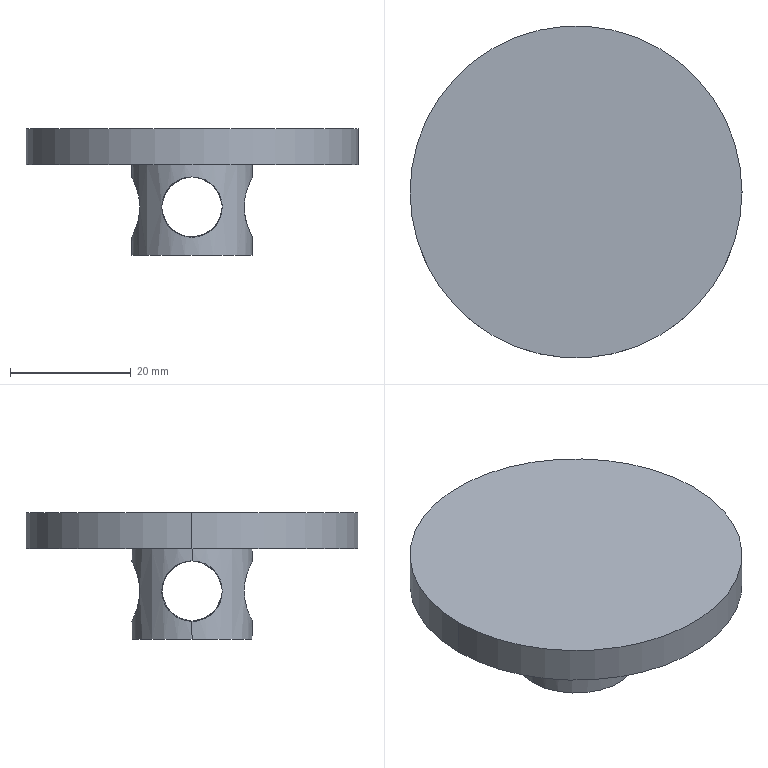Part | SolidWorks | features ICE 2, CirPattern 1, MBimport 1 | 1 solid | 15 faces | box 55 x 55 x 21 mm | volume 16595 mm3 | spline 8 | cylinder 4 | plane 3 | commonest cylinder face diameters 20 x2 55 x2